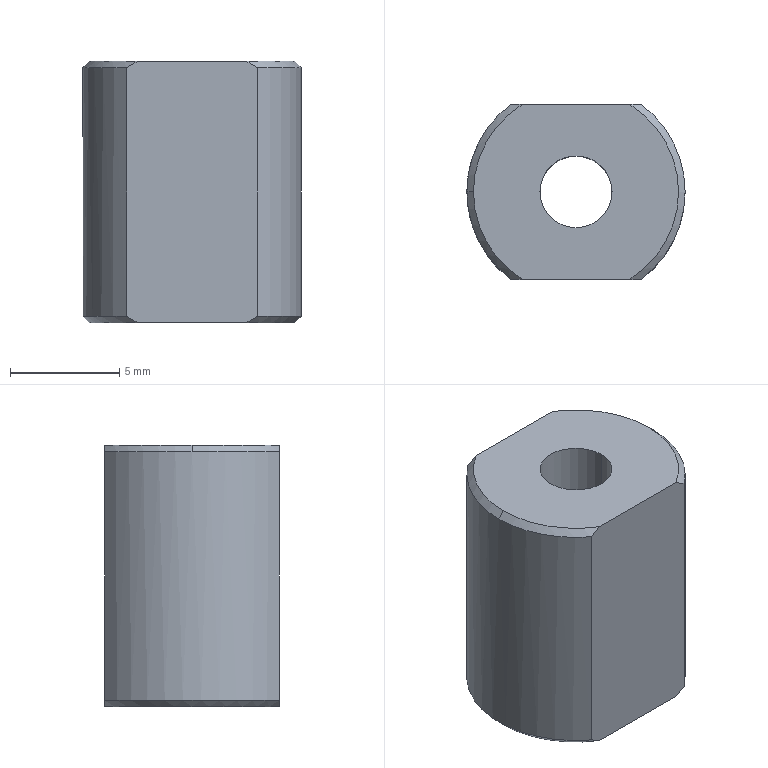Part | NX | 1 solid | 17 faces | box 10 x 8 x 12 mm | volume 738.555 mm3 | cone 8 | cylinder 5 | plane 4 | commonest cylinder face diameters 10 x3 3.3 x2
STEP:
#1=CARTESIAN_POINT('',(5.,0.,39.2));
#2=VERTEX_POINT('',#1);
#3=CARTESIAN_POINT('',(5.,0.,50.6));
#4=VERTEX_POINT('',#3);
#5=CARTESIAN_POINT('',(5.,0.,38.9));
#6=DIRECTION('',(0.,0.,1.));
#7=VECTOR('',#6,1000.);
#8=LINE('',#5,#7);
#9=EDGE_CURVE('',#2,#4,#8,.T.);
#10=ORIENTED_EDGE('',*,*,#9,.F.);
#11=CARTESIAN_POINT('',(3.,4.,39.2));
#12=VERTEX_POINT('',#11);
#13=CARTESIAN_POINT('',(0.,0.,39.2));
#14=DIRECTION('',(0.,0.,1.));
#15=DIRECTION('',(1.,0.,0.));
#16=AXIS2_PLACEMENT_3D('',#13,#14,#15);
#17=CIRCLE('',#16,5.);
#18=EDGE_CURVE('',#2,#12,#17,.T.);
#19=ORIENTED_EDGE('',*,*,#18,.T.);
#20=CARTESIAN_POINT('',(3.,4.,50.6));
#21=VERTEX_POINT('',#20);
#22=CARTESIAN_POINT('',(3.,4.,38.9));
#23=DIRECTION('',(0.,0.,1.));
#24=VECTOR('',#23,1000.);
#25=LINE('',#22,#24);
#26=EDGE_CURVE('',#12,#21,#25,.T.);
#27=ORIENTED_EDGE('',*,*,#26,.T.);
#28=CARTESIAN_POINT('',(0.,0.,50.6));
#29=DIRECTION('',(0.,0.,1.));
#30=DIRECTION('',(1.,0.,0.));
#31=AXIS2_PLACEMENT_3D('',#28,#29,#30);
#32=CIRCLE('',#31,5.);
#33=EDGE_CURVE('',#4,#21,#32,.T.);
#34=ORIENTED_EDGE('',*,*,#33,.F.);
#35=EDGE_LOOP('',(#10,#19,#27,#34));
#36=FACE_BOUND('',#35,.T.);
#37=CARTESIAN_POINT('',(0.,0.,38.9));
#38=DIRECTION('',(0.,0.,1.));
#39=DIRECTION('',(1.,0.,0.));
#40=AXIS2_PLACEMENT_3D('',#37,#38,#39);
#41=CYLINDRICAL_SURFACE('',#40,5.);
#42=ADVANCED_FACE('',(#36),#41,.T.);
#43=CARTESIAN_POINT('',(-3.,-4.,39.2));
#44=VERTEX_POINT('',#43);
#45=CARTESIAN_POINT('',(-3.,-4.,50.6));
#46=VERTEX_POINT('',#45);
#47=CARTESIAN_POINT('',(-3.,-4.,38.9));
#48=DIRECTION('',(0.,0.,1.));
#49=VECTOR('',#48,1000.);
#50=LINE('',#47,#49);
#51=EDGE_CURVE('',#44,#46,#50,.T.);
#52=ORIENTED_EDGE('',*,*,#51,.T.);
#53=CARTESIAN_POINT('',(-5.,0.,50.6));
#54=VERTEX_POINT('',#53);
#55=CARTESIAN_POINT('',(0.,0.,50.6));
#56=DIRECTION('',(0.,0.,1.));
#57=DIRECTION('',(1.,0.,0.));
#58=AXIS2_PLACEMENT_3D('',#55,#56,#57);
#59=CIRCLE('',#58,5.);
#60=EDGE_CURVE('',#54,#46,#59,.T.);
#61=ORIENTED_EDGE('',*,*,#60,.F.);
#62=CARTESIAN_POINT('',(-3.,4.,50.6));
#63=VERTEX_POINT('',#62);
#64=CARTESIAN_POINT('',(0.,0.,50.6));
#65=DIRECTION('',(0.,0.,1.));
#66=DIRECTION('',(1.,0.,0.));
#67=AXIS2_PLACEMENT_3D('',#64,#65,#66);
#68=CIRCLE('',#67,5.);
#69=EDGE_CURVE('',#63,#54,#68,.T.);
#70=ORIENTED_EDGE('',*,*,#69,.F.);
#71=CARTESIAN_POINT('',(-3.,4.,39.2));
#72=VERTEX_POINT('',#71);
#73=CARTESIAN_POINT('',(-3.,4.,38.9));
#74=DIRECTION('',(0.,0.,1.));
#75=VECTOR('',#74,1000.);
#76=LINE('',#73,#75);
#77=EDGE_CURVE('',#72,#63,#76,.T.);
#78=ORIENTED_EDGE('',*,*,#77,.F.);
#79=CARTESIAN_POINT('',(0.,0.,39.2));
#80=DIRECTION('',(0.,0.,1.));
#81=DIRECTION('',(1.,0.,0.));
#82=AXIS2_PLACEMENT_3D('',#79,#80,#81);
#83=CIRCLE('',#82,5.);
#84=EDGE_CURVE('',#72,#44,#83,.T.);
#85=ORIENTED_EDGE('',*,*,#84,.T.);
#86=EDGE_LOOP('',(#52,#61,#70,#78,#85));
#87=FACE_BOUND('',#86,.T.);
#88=CARTESIAN_POINT('',(0.,0.,38.9));
#89=DIRECTION('',(0.,0.,1.));
#90=DIRECTION('',(1.,0.,0.));
#91=AXIS2_PLACEMENT_3D('',#88,#89,#90);
#92=CYLINDRICAL_SURFACE('',#91,5.);
#93=ADVANCED_FACE('',(#87),#92,.T.);
#94=CARTESIAN_POINT('',(2.468,-4.,50.9));
#95=VERTEX_POINT('',#94);
#96=CARTESIAN_POINT('',(2.468,4.,50.9));
#97=VERTEX_POINT('',#96);
#98=CARTESIAN_POINT('',(0.,0.,50.9));
#99=DIRECTION('',(0.,0.,1.));
#100=DIRECTION('',(1.,0.,0.));
#101=AXIS2_PLACEMENT_3D('',#98,#99,#100);
#102=CIRCLE('',#101,4.7);
#103=EDGE_CURVE('',#95,#97,#102,.T.);
#104=ORIENTED_EDGE('',*,*,#103,.T.);
#105=CARTESIAN_POINT('',(-2.468,4.,50.9));
#106=VERTEX_POINT('',#105);
#107=CARTESIAN_POINT('',(-2.871,4.,50.9));
#108=DIRECTION('',(1.,0.,0.));
#109=VECTOR('',#108,1000.);
#110=LINE('',#107,#109);
#111=EDGE_CURVE('',#106,#97,#110,.T.);
#112=ORIENTED_EDGE('',*,*,#111,.F.);
#113=CARTESIAN_POINT('',(-4.7,0.,50.9));
#114=VERTEX_POINT('',#113);
#115=CARTESIAN_POINT('',(0.,0.,50.9));
#116=DIRECTION('',(0.,0.,1.));
#117=DIRECTION('',(1.,0.,0.));
#118=AXIS2_PLACEMENT_3D('',#115,#116,#117);
#119=CIRCLE('',#118,4.7);
#120=EDGE_CURVE('',#106,#114,#119,.T.);
#121=ORIENTED_EDGE('',*,*,#120,.T.);
#122=CARTESIAN_POINT('',(-2.468,-4.,50.9));
#123=VERTEX_POINT('',#122);
#124=CARTESIAN_POINT('',(0.,0.,50.9));
#125=DIRECTION('',(0.,0.,1.));
#126=DIRECTION('',(1.,0.,0.));
#127=AXIS2_PLACEMENT_3D('',#124,#125,#126);
#128=CIRCLE('',#127,4.7);
#129=EDGE_CURVE('',#114,#123,#128,.T.);
#130=ORIENTED_EDGE('',*,*,#129,.T.);
#131=CARTESIAN_POINT('',(-2.871,-4.,50.9));
#132=DIRECTION('',(-1.,0.,0.));
#133=VECTOR('',#132,1000.);
#134=LINE('',#131,#133);
#135=EDGE_CURVE('',#95,#123,#134,.T.);
#136=ORIENTED_EDGE('',*,*,#135,.F.);
#137=EDGE_LOOP('',(#104,#112,#121,#130,#136));
#138=FACE_BOUND('',#137,.T.);
#139=CARTESIAN_POINT('',(1.65,0.,50.9));
#140=VERTEX_POINT('',#139);
#141=CARTESIAN_POINT('',(-1.65,0.,50.9));
#142=VERTEX_POINT('',#141);
#143=CARTESIAN_POINT('',(0.,0.,50.9));
#144=DIRECTION('',(0.,0.,-1.));
#145=DIRECTION('',(-1.,0.,0.));
#146=AXIS2_PLACEMENT_3D('',#143,#144,#145);
#147=CIRCLE('',#146,1.65);
#148=EDGE_CURVE('',#140,#142,#147,.T.);
#149=ORIENTED_EDGE('',*,*,#148,.T.);
#150=CARTESIAN_POINT('',(0.,0.,50.9));
#151=DIRECTION('',(0.,0.,-1.));
#152=DIRECTION('',(-1.,0.,0.));
#153=AXIS2_PLACEMENT_3D('',#150,#151,#152);
#154=CIRCLE('',#153,1.65);
#155=EDGE_CURVE('',#142,#140,#154,.T.);
#156=ORIENTED_EDGE('',*,*,#155,.T.);
#157=EDGE_LOOP('',(#149,#156));
#158=FACE_BOUND('',#157,.T.);
#159=CARTESIAN_POINT('',(-2.871,0.,50.9));
#160=DIRECTION('',(0.,0.,1.));
#161=DIRECTION('',(1.,0.,0.));
#162=AXIS2_PLACEMENT_3D('',#159,#160,#161);
#163=PLANE('',#162);
#164=ADVANCED_FACE('',(#138,#158),#163,.T.);
#165=CARTESIAN_POINT('',(1.65,0.,39.284));
#166=VERTEX_POINT('',#165);
#167=CARTESIAN_POINT('',(-1.65,0.,39.284));
#168=VERTEX_POINT('',#167);
#169=CARTESIAN_POINT('',(0.,0.,39.284));
#170=DIRECTION('',(0.,0.,-1.));
#171=DIRECTION('',(-1.,0.,0.));
#172=AXIS2_PLACEMENT_3D('',#169,#170,#171);
#173=CIRCLE('',#172,1.65);
#174=EDGE_CURVE('',#166,#168,#173,.T.);
#175=ORIENTED_EDGE('',*,*,#174,.T.);
#176=CARTESIAN_POINT('',(-1.65,0.,38.9));
#177=DIRECTION('',(0.,0.,-1.));
#178=VECTOR('',#177,1000.);
#179=LINE('',#176,#178);
#180=EDGE_CURVE('',#168,#142,#179,.F.);
#181=ORIENTED_EDGE('',*,*,#180,.T.);
#182=ORIENTED_EDGE('',*,*,#148,.F.);
#183=CARTESIAN_POINT('',(1.65,0.,38.9));
#184=DIRECTION('',(0.,0.,-1.));
#185=VECTOR('',#184,1000.);
#186=LINE('',#183,#185);
#187=EDGE_CURVE('',#166,#140,#186,.F.);
#188=ORIENTED_EDGE('',*,*,#187,.F.);
#189=EDGE_LOOP('',(#175,#181,#182,#188));
#190=FACE_BOUND('',#189,.T.);
#191=CARTESIAN_POINT('',(0.,0.,38.9));
#192=DIRECTION('',(0.,0.,-1.));
#193=DIRECTION('',(-1.,0.,0.));
#194=AXIS2_PLACEMENT_3D('',#191,#192,#193);
#195=CYLINDRICAL_SURFACE('',#194,1.65);
#196=ADVANCED_FACE('',(#190),#195,.F.);
#197=ORIENTED_EDGE('',*,*,#174,.F.);
#198=CARTESIAN_POINT('',(2.315,0.,38.9));
#199=VERTEX_POINT('',#198);
#200=CARTESIAN_POINT('',(1.65,0.,39.284));
#201=DIRECTION('',(0.866,0.,-0.5));
#202=VECTOR('',#201,1000.);
#203=LINE('',#200,#202);
#204=EDGE_CURVE('',#199,#166,#203,.F.);
#205=ORIENTED_EDGE('',*,*,#204,.F.);
#206=CARTESIAN_POINT('',(-2.315,0.,38.9));
#207=VERTEX_POINT('',#206);
#208=CARTESIAN_POINT('',(0.,0.,38.9));
#209=DIRECTION('',(0.,0.,-1.));
#210=DIRECTION('',(-1.,0.,0.));
#211=AXIS2_PLACEMENT_3D('',#208,#209,#210);
#212=CIRCLE('',#211,2.315);
#213=EDGE_CURVE('',#199,#207,#212,.T.);
#214=ORIENTED_EDGE('',*,*,#213,.T.);
#215=CARTESIAN_POINT('',(-1.65,0.,39.284));
#216=DIRECTION('',(-0.866,0.,-0.5));
#217=VECTOR('',#216,1000.);
#218=LINE('',#215,#217);
#219=EDGE_CURVE('',#207,#168,#218,.F.);
#220=ORIENTED_EDGE('',*,*,#219,.T.);
#221=EDGE_LOOP('',(#197,#205,#214,#220));
#222=FACE_BOUND('',#221,.T.);
#223=CARTESIAN_POINT('',(0.,0.,39.284));
#224=DIRECTION('',(0.,0.,-1.));
#225=DIRECTION('',(-1.,0.,0.));
#226=AXIS2_PLACEMENT_3D('',#223,#224,#225);
#227=CONICAL_SURFACE('',#226,1.65,1.047);
#228=ADVANCED_FACE('',(#222),#227,.F.);
#229=ORIENTED_EDGE('',*,*,#51,.F.);
#230=CARTESIAN_POINT('',(-2.468,-4.,38.9));
#231=VERTEX_POINT('',#230);
#232=CARTESIAN_POINT('',(-3.,-4.,39.2));
#233=CARTESIAN_POINT('',(-2.956,-4.,39.174));
#234=CARTESIAN_POINT('',(-2.913,-4.,39.148));
#235=CARTESIAN_POINT('',(-2.869,-4.,39.122));
#236=CARTESIAN_POINT('',(-2.825,-4.,39.097));
#237=CARTESIAN_POINT('',(-2.781,-4.,39.071));
#238=CARTESIAN_POINT('',(-2.736,-4.,39.046));
#239=CARTESIAN_POINT('',(-2.692,-4.,39.021));
#240=CARTESIAN_POINT('',(-2.647,-4.,38.997));
#241=CARTESIAN_POINT('',(-2.603,-4.,38.972));
#242=CARTESIAN_POINT('',(-2.558,-4.,38.948));
#243=CARTESIAN_POINT('',(-2.513,-4.,38.924));
#244=CARTESIAN_POINT('',(-2.468,-4.,38.9));
#245=B_SPLINE_CURVE_WITH_KNOTS('',3,(#232,#233,#234,#235,#236,#237,#238,#239,#240,#241,#242,#243,#244),.UNSPECIFIED.,.F.,.F.,(4,3,3,3,4),(0.,0.1525,0.3051,0.458,0.611),.UNSPECIFIED.);
#246=EDGE_CURVE('',#44,#231,#245,.T.);
#247=ORIENTED_EDGE('',*,*,#246,.T.);
#248=CARTESIAN_POINT('',(2.468,-4.,38.9));
#249=VERTEX_POINT('',#248);
#250=CARTESIAN_POINT('',(-2.871,-4.,38.9));
#251=DIRECTION('',(-1.,0.,0.));
#252=VECTOR('',#251,1000.);
#253=LINE('',#250,#252);
#254=EDGE_CURVE('',#249,#231,#253,.T.);
#255=ORIENTED_EDGE('',*,*,#254,.F.);
#256=CARTESIAN_POINT('',(3.,-4.,39.2));
#257=VERTEX_POINT('',#256);
#258=CARTESIAN_POINT('',(2.468,-4.,38.9));
#259=CARTESIAN_POINT('',(2.513,-4.,38.924));
#260=CARTESIAN_POINT('',(2.558,-4.,38.948));
#261=CARTESIAN_POINT('',(2.602,-4.,38.972));
#262=CARTESIAN_POINT('',(2.647,-4.,38.996));
#263=CARTESIAN_POINT('',(2.692,-4.,39.021));
#264=CARTESIAN_POINT('',(2.736,-4.,39.046));
#265=CARTESIAN_POINT('',(2.78,-4.,39.071));
#266=CARTESIAN_POINT('',(2.824,-4.,39.097));
#267=CARTESIAN_POINT('',(2.868,-4.,39.122));
#268=CARTESIAN_POINT('',(2.912,-4.,39.148));
#269=CARTESIAN_POINT('',(2.956,-4.,39.174));
#270=CARTESIAN_POINT('',(3.,-4.,39.2));
#271=B_SPLINE_CURVE_WITH_KNOTS('',3,(#258,#259,#260,#261,#262,#263,#264,#265,#266,#267,#268,#269,#270),.UNSPECIFIED.,.F.,.F.,(4,3,3,3,4),(0.,0.1527,0.3054,0.4582,0.611),.UNSPECIFIED.);
#272=EDGE_CURVE('',#249,#257,#271,.T.);
#273=ORIENTED_EDGE('',*,*,#272,.T.);
#274=CARTESIAN_POINT('',(3.,-4.,50.6));
#275=VERTEX_POINT('',#274);
#276=CARTESIAN_POINT('',(3.,-4.,38.9));
#277=DIRECTION('',(0.,0.,1.));
#278=VECTOR('',#277,1000.);
#279=LINE('',#276,#278);
#280=EDGE_CURVE('',#257,#275,#279,.T.);
#281=ORIENTED_EDGE('',*,*,#280,.T.);
#282=CARTESIAN_POINT('',(3.,-4.,50.6));
#283=CARTESIAN_POINT('',(2.956,-4.,50.626));
#284=CARTESIAN_POINT('',(2.912,-4.,50.652));
#285=CARTESIAN_POINT('',(2.868,-4.,50.678));
#286=CARTESIAN_POINT('',(2.824,-4.,50.703));
#287=CARTESIAN_POINT('',(2.78,-4.,50.729));
#288=CARTESIAN_POINT('',(2.736,-4.,50.754));
#289=CARTESIAN_POINT('',(2.692,-4.,50.779));
#290=CARTESIAN_POINT('',(2.647,-4.,50.804));
#291=CARTESIAN_POINT('',(2.602,-4.,50.828));
#292=CARTESIAN_POINT('',(2.558,-4.,50.852));
#293=CARTESIAN_POINT('',(2.513,-4.,50.876));
#294=CARTESIAN_POINT('',(2.468,-4.,50.9));
#295=B_SPLINE_CURVE_WITH_KNOTS('',3,(#282,#283,#284,#285,#286,#287,#288,#289,#290,#291,#292,#293,#294),.UNSPECIFIED.,.F.,.F.,(4,3,3,3,4),(0.,0.1528,0.3056,0.4583,0.611),.UNSPECIFIED.);
#296=EDGE_CURVE('',#275,#95,#295,.T.);
#297=ORIENTED_EDGE('',*,*,#296,.T.);
#298=ORIENTED_EDGE('',*,*,#135,.T.);
#299=CARTESIAN_POINT('',(-2.468,-4.,50.9));
#300=CARTESIAN_POINT('',(-2.513,-4.,50.876));
#301=CARTESIAN_POINT('',(-2.558,-4.,50.852));
#302=CARTESIAN_POINT('',(-2.603,-4.,50.828));
#303=CARTESIAN_POINT('',(-2.647,-4.,50.803));
#304=CARTESIAN_POINT('',(-2.692,-4.,50.779));
#305=CARTESIAN_POINT('',(-2.736,-4.,50.754));
#306=CARTESIAN_POINT('',(-2.781,-4.,50.729));
#307=CARTESIAN_POINT('',(-2.825,-4.,50.703));
#308=CARTESIAN_POINT('',(-2.869,-4.,50.678));
#309=CARTESIAN_POINT('',(-2.913,-4.,50.652));
#310=CARTESIAN_POINT('',(-2.956,-4.,50.626));
#311=CARTESIAN_POINT('',(-3.,-4.,50.6));
#312=B_SPLINE_CURVE_WITH_KNOTS('',3,(#299,#300,#301,#302,#303,#304,#305,#306,#307,#308,#309,#310,#311),.UNSPECIFIED.,.F.,.F.,(4,3,3,3,4),(0.,0.153,0.3057,0.4584,0.611),.UNSPECIFIED.);
#313=EDGE_CURVE('',#123,#46,#312,.T.);
#314=ORIENTED_EDGE('',*,*,#313,.T.);
#315=EDGE_LOOP('',(#229,#247,#255,#273,#281,#297,#298,#314));
#316=FACE_BOUND('',#315,.T.);
#317=CARTESIAN_POINT('',(7.4,-4.,52.1));
#318=DIRECTION('',(0.,1.,0.));
#319=DIRECTION('',(1.,0.,0.));
#320=AXIS2_PLACEMENT_3D('',#317,#318,#319);
#321=PLANE('',#320);
#322=ADVANCED_FACE('',(#316),#321,.F.);
#323=ORIENTED_EDGE('',*,*,#26,.F.);
#324=CARTESIAN_POINT('',(2.468,4.,38.9));
#325=VERTEX_POINT('',#324);
#326=CARTESIAN_POINT('',(3.,4.,39.2));
#327=CARTESIAN_POINT('',(2.956,4.,39.174));
#328=CARTESIAN_POINT('',(2.913,4.,39.148));
#329=CARTESIAN_POINT('',(2.869,4.,39.122));
#330=CARTESIAN_POINT('',(2.825,4.,39.097));
#331=CARTESIAN_POINT('',(2.781,4.,39.071));
#332=CARTESIAN_POINT('',(2.736,4.,39.046));
#333=CARTESIAN_POINT('',(2.692,4.,39.021));
#334=CARTESIAN_POINT('',(2.647,4.,38.997));
#335=CARTESIAN_POINT('',(2.603,4.,38.972));
#336=CARTESIAN_POINT('',(2.558,4.,38.948));
#337=CARTESIAN_POINT('',(2.513,4.,38.924));
#338=CARTESIAN_POINT('',(2.468,4.,38.9));
#339=B_SPLINE_CURVE_WITH_KNOTS('',3,(#326,#327,#328,#329,#330,#331,#332,#333,#334,#335,#336,#337,#338),.UNSPECIFIED.,.F.,.F.,(4,3,3,3,4),(0.,0.1525,0.3051,0.458,0.611),.UNSPECIFIED.);
#340=EDGE_CURVE('',#12,#325,#339,.T.);
#341=ORIENTED_EDGE('',*,*,#340,.T.);
#342=CARTESIAN_POINT('',(-2.468,4.,38.9));
#343=VERTEX_POINT('',#342);
#344=CARTESIAN_POINT('',(-2.871,4.,38.9));
#345=DIRECTION('',(1.,0.,0.));
#346=VECTOR('',#345,1000.);
#347=LINE('',#344,#346);
#348=EDGE_CURVE('',#343,#325,#347,.T.);
#349=ORIENTED_EDGE('',*,*,#348,.F.);
#350=CARTESIAN_POINT('',(-2.468,4.,38.9));
#351=CARTESIAN_POINT('',(-2.513,4.,38.924));
#352=CARTESIAN_POINT('',(-2.558,4.,38.948));
#353=CARTESIAN_POINT('',(-2.602,4.,38.972));
#354=CARTESIAN_POINT('',(-2.647,4.,38.996));
#355=CARTESIAN_POINT('',(-2.692,4.,39.021));
#356=CARTESIAN_POINT('',(-2.736,4.,39.046));
#357=CARTESIAN_POINT('',(-2.78,4.,39.071));
#358=CARTESIAN_POINT('',(-2.824,4.,39.097));
#359=CARTESIAN_POINT('',(-2.868,4.,39.122));
#360=CARTESIAN_POINT('',(-2.912,4.,39.148));
#361=CARTESIAN_POINT('',(-2.956,4.,39.174));
#362=CARTESIAN_POINT('',(-3.,4.,39.2));
#363=B_SPLINE_CURVE_WITH_KNOTS('',3,(#350,#351,#352,#353,#354,#355,#356,#357,#358,#359,#360,#361,#362),.UNSPECIFIED.,.F.,.F.,(4,3,3,3,4),(0.,0.1527,0.3054,0.4582,0.611),.UNSPECIFIED.);
#364=EDGE_CURVE('',#343,#72,#363,.T.);
#365=ORIENTED_EDGE('',*,*,#364,.T.);
#366=ORIENTED_EDGE('',*,*,#77,.T.);
#367=CARTESIAN_POINT('',(-3.,4.,50.6));
#368=CARTESIAN_POINT('',(-2.956,4.,50.626));
#369=CARTESIAN_POINT('',(-2.912,4.,50.652));
#370=CARTESIAN_POINT('',(-2.868,4.,50.678));
#371=CARTESIAN_POINT('',(-2.824,4.,50.703));
#372=CARTESIAN_POINT('',(-2.78,4.,50.729));
#373=CARTESIAN_POINT('',(-2.736,4.,50.754));
#374=CARTESIAN_POINT('',(-2.692,4.,50.779));
#375=CARTESIAN_POINT('',(-2.647,4.,50.804));
#376=CARTESIAN_POINT('',(-2.602,4.,50.828));
#377=CARTESIAN_POINT('',(-2.558,4.,50.852));
#378=CARTESIAN_POINT('',(-2.513,4.,50.876));
#379=CARTESIAN_POINT('',(-2.468,4.,50.9));
#380=B_SPLINE_CURVE_WITH_KNOTS('',3,(#367,#368,#369,#370,#371,#372,#373,#374,#375,#376,#377,#378,#379),.UNSPECIFIED.,.F.,.F.,(4,3,3,3,4),(0.,0.1528,0.3056,0.4583,0.611),.UNSPECIFIED.);
#381=EDGE_CURVE('',#63,#106,#380,.T.);
#382=ORIENTED_EDGE('',*,*,#381,.T.);
#383=ORIENTED_EDGE('',*,*,#111,.T.);
#384=CARTESIAN_POINT('',(2.468,4.,50.9));
#385=CARTESIAN_POINT('',(2.513,4.,50.876));
#386=CARTESIAN_POINT('',(2.558,4.,50.852));
#387=CARTESIAN_POINT('',(2.603,4.,50.828));
#388=CARTESIAN_POINT('',(2.647,4.,50.803));
#389=CARTESIAN_POINT('',(2.692,4.,50.779));
#390=CARTESIAN_POINT('',(2.736,4.,50.754));
#391=CARTESIAN_POINT('',(2.781,4.,50.729));
#392=CARTESIAN_POINT('',(2.825,4.,50.703));
#393=CARTESIAN_POINT('',(2.869,4.,50.678));
#394=CARTESIAN_POINT('',(2.913,4.,50.652));
#395=CARTESIAN_POINT('',(2.956,4.,50.626));
#396=CARTESIAN_POINT('',(3.,4.,50.6));
#397=B_SPLINE_CURVE_WITH_KNOTS('',3,(#384,#385,#386,#387,#388,#389,#390,#391,#392,#393,#394,#395,#396),.UNSPECIFIED.,.F.,.F.,(4,3,3,3,4),(0.,0.153,0.3058,0.4584,0.611),.UNSPECIFIED.);
#398=EDGE_CURVE('',#97,#21,#397,.T.);
#399=ORIENTED_EDGE('',*,*,#398,.T.);
#400=EDGE_LOOP('',(#323,#341,#349,#365,#366,#382,#383,#399));
#401=FACE_BOUND('',#400,.T.);
#402=CARTESIAN_POINT('',(-5.9,4.,52.1));
#403=DIRECTION('',(0.,-1.,0.));
#404=DIRECTION('',(0.,0.,-1.));
#405=AXIS2_PLACEMENT_3D('',#402,#403,#404);
#406=PLANE('',#405);
#407=ADVANCED_FACE('',(#401),#406,.F.);
#408=CARTESIAN_POINT('',(-4.7,0.,50.9));
#409=DIRECTION('',(-0.7071,0.,-0.7071));
#410=VECTOR('',#409,1000.);
#411=LINE('',#408,#410);
#412=EDGE_CURVE('',#114,#54,#411,.T.);
#413=ORIENTED_EDGE('',*,*,#412,.F.);
#414=ORIENTED_EDGE('',*,*,#120,.F.);
#415=ORIENTED_EDGE('',*,*,#381,.F.);
#416=ORIENTED_EDGE('',*,*,#69,.T.);
#417=EDGE_LOOP('',(#413,#414,#415,#416));
#418=FACE_BOUND('',#417,.T.);
#419=CARTESIAN_POINT('',(0.,0.,50.9));
#420=DIRECTION('',(0.,0.,-1.));
#421=DIRECTION('',(-1.,0.,0.));
#422=AXIS2_PLACEMENT_3D('',#419,#420,#421);
#423=CONICAL_SURFACE('',#422,4.7,0.7854);
#424=ADVANCED_FACE('',(#418),#423,.T.);
#425=ORIENTED_EDGE('',*,*,#103,.F.);
#426=ORIENTED_EDGE('',*,*,#296,.F.);
#427=CARTESIAN_POINT('',(0.,0.,50.6));
#428=DIRECTION('',(0.,0.,1.));
#429=DIRECTION('',(1.,0.,0.));
#430=AXIS2_PLACEMENT_3D('',#427,#428,#429);
#431=CIRCLE('',#430,5.);
#432=EDGE_CURVE('',#275,#4,#431,.T.);
#433=ORIENTED_EDGE('',*,*,#432,.T.);
#434=ORIENTED_EDGE('',*,*,#33,.T.);
#435=ORIENTED_EDGE('',*,*,#398,.F.);
#436=EDGE_LOOP('',(#425,#426,#433,#434,#435));
#437=FACE_BOUND('',#436,.T.);
#438=CARTESIAN_POINT('',(0.,0.,50.9));
#439=DIRECTION('',(0.,0.,-1.));
#440=DIRECTION('',(-1.,0.,0.));
#441=AXIS2_PLACEMENT_3D('',#438,#439,#440);
#442=CONICAL_SURFACE('',#441,4.7,0.7854);
#443=ADVANCED_FACE('',(#437),#442,.T.);
#444=ORIENTED_EDGE('',*,*,#180,.F.);
#445=CARTESIAN_POINT('',(0.,0.,39.284));
#446=DIRECTION('',(0.,0.,-1.));
#447=DIRECTION('',(-1.,0.,0.));
#448=AXIS2_PLACEMENT_3D('',#445,#446,#447);
#449=CIRCLE('',#448,1.65);
#450=EDGE_CURVE('',#168,#166,#449,.T.);
#451=ORIENTED_EDGE('',*,*,#450,.T.);
#452=ORIENTED_EDGE('',*,*,#187,.T.);
#453=ORIENTED_EDGE('',*,*,#155,.F.);
#454=EDGE_LOOP('',(#444,#451,#452,#453));
#455=FACE_BOUND('',#454,.T.);
#456=CARTESIAN_POINT('',(0.,0.,38.9));
#457=DIRECTION('',(0.,0.,-1.));
#458=DIRECTION('',(-1.,0.,0.));
#459=AXIS2_PLACEMENT_3D('',#456,#457,#458);
#460=CYLINDRICAL_SURFACE('',#459,1.65);
#461=ADVANCED_FACE('',(#455),#460,.F.);
#462=ORIENTED_EDGE('',*,*,#219,.F.);
#463=CARTESIAN_POINT('',(0.,0.,38.9));
#464=DIRECTION('',(0.,0.,-1.));
#465=DIRECTION('',(-1.,0.,0.));
#466=AXIS2_PLACEMENT_3D('',#463,#464,#465);
#467=CIRCLE('',#466,2.315);
#468=EDGE_CURVE('',#207,#199,#467,.T.);
#469=ORIENTED_EDGE('',*,*,#468,.T.);
#470=ORIENTED_EDGE('',*,*,#204,.T.);
#471=ORIENTED_EDGE('',*,*,#450,.F.);
#472=EDGE_LOOP('',(#462,#469,#470,#471));
#473=FACE_BOUND('',#472,.T.);
#474=CARTESIAN_POINT('',(0.,0.,39.284));
#475=DIRECTION('',(0.,0.,-1.));
#476=DIRECTION('',(-1.,0.,0.));
#477=AXIS2_PLACEMENT_3D('',#474,#475,#476);
#478=CONICAL_SURFACE('',#477,1.65,1.047);
#479=ADVANCED_FACE('',(#473),#478,.F.);
#480=CARTESIAN_POINT('',(0.,0.,38.9));
#481=DIRECTION('',(0.,0.,1.));
#482=DIRECTION('',(1.,0.,0.));
#483=AXIS2_PLACEMENT_3D('',#480,#481,#482);
#484=CIRCLE('',#483,4.7);
#485=EDGE_CURVE('',#343,#231,#484,.T.);
#486=ORIENTED_EDGE('',*,*,#485,.F.);
#487=ORIENTED_EDGE('',*,*,#348,.T.);
#488=CARTESIAN_POINT('',(4.7,0.,38.9));
#489=VERTEX_POINT('',#488);
#490=CARTESIAN_POINT('',(0.,0.,38.9));
#491=DIRECTION('',(0.,0.,1.));
#492=DIRECTION('',(1.,0.,0.));
#493=AXIS2_PLACEMENT_3D('',#490,#491,#492);
#494=CIRCLE('',#493,4.7);
#495=EDGE_CURVE('',#489,#325,#494,.T.);
#496=ORIENTED_EDGE('',*,*,#495,.F.);
#497=CARTESIAN_POINT('',(0.,0.,38.9));
#498=DIRECTION('',(0.,0.,1.));
#499=DIRECTION('',(1.,0.,0.));
#500=AXIS2_PLACEMENT_3D('',#497,#498,#499);
#501=CIRCLE('',#500,4.7);
#502=EDGE_CURVE('',#249,#489,#501,.T.);
#503=ORIENTED_EDGE('',*,*,#502,.F.);
#504=ORIENTED_EDGE('',*,*,#254,.T.);
#505=EDGE_LOOP('',(#486,#487,#496,#503,#504));
#506=FACE_BOUND('',#505,.T.);
#507=ORIENTED_EDGE('',*,*,#213,.F.);
#508=ORIENTED_EDGE('',*,*,#468,.F.);
#509=EDGE_LOOP('',(#507,#508));
#510=FACE_BOUND('',#509,.T.);
#511=CARTESIAN_POINT('',(-2.871,0.,38.9));
#512=DIRECTION('',(0.,0.,1.));
#513=DIRECTION('',(1.,0.,0.));
#514=AXIS2_PLACEMENT_3D('',#511,#512,#513);
#515=PLANE('',#514);
#516=ADVANCED_FACE('',(#506,#510),#515,.F.);
#517=CARTESIAN_POINT('',(4.7,0.,38.9));
#518=DIRECTION('',(0.7071,0.,0.7071));
#519=VECTOR('',#518,1000.);
#520=LINE('',#517,#519);
#521=EDGE_CURVE('',#489,#2,#520,.T.);
#522=ORIENTED_EDGE('',*,*,#521,.F.);
#523=ORIENTED_EDGE('',*,*,#495,.T.);
#524=ORIENTED_EDGE('',*,*,#340,.F.);
#525=ORIENTED_EDGE('',*,*,#18,.F.);
#526=EDGE_LOOP('',(#522,#523,#524,#525));
#527=FACE_BOUND('',#526,.T.);
#528=CARTESIAN_POINT('',(0.,0.,38.9));
#529=DIRECTION('',(0.,0.,1.));
#530=DIRECTION('',(1.,0.,0.));
#531=AXIS2_PLACEMENT_3D('',#528,#529,#530);
#532=CONICAL_SURFACE('',#531,4.7,0.7854);
#533=ADVANCED_FACE('',(#527),#532,.T.);
#534=ORIENTED_EDGE('',*,*,#485,.T.);
#535=ORIENTED_EDGE('',*,*,#246,.F.);
#536=ORIENTED_EDGE('',*,*,#84,.F.);
#537=ORIENTED_EDGE('',*,*,#364,.F.);
#538=EDGE_LOOP('',(#534,#535,#536,#537));
#539=FACE_BOUND('',#538,.T.);
#540=CARTESIAN_POINT('',(0.,0.,38.9));
#541=DIRECTION('',(0.,0.,1.));
#542=DIRECTION('',(1.,0.,0.));
#543=AXIS2_PLACEMENT_3D('',#540,#541,#542);
#544=CONICAL_SURFACE('',#543,4.7,0.7854);
#545=ADVANCED_FACE('',(#539),#544,.T.);
#546=ORIENTED_EDGE('',*,*,#502,.T.);
#547=ORIENTED_EDGE('',*,*,#521,.T.);
#548=CARTESIAN_POINT('',(0.,0.,39.2));
#549=DIRECTION('',(0.,0.,1.));
#550=DIRECTION('',(1.,0.,0.));
#551=AXIS2_PLACEMENT_3D('',#548,#549,#550);
#552=CIRCLE('',#551,5.);
#553=EDGE_CURVE('',#257,#2,#552,.T.);
#554=ORIENTED_EDGE('',*,*,#553,.F.);
#555=ORIENTED_EDGE('',*,*,#272,.F.);
#556=EDGE_LOOP('',(#546,#547,#554,#555));
#557=FACE_BOUND('',#556,.T.);
#558=CARTESIAN_POINT('',(0.,0.,38.9));
#559=DIRECTION('',(0.,0.,1.));
#560=DIRECTION('',(1.,0.,0.));
#561=AXIS2_PLACEMENT_3D('',#558,#559,#560);
#562=CONICAL_SURFACE('',#561,4.7,0.7854);
#563=ADVANCED_FACE('',(#557),#562,.T.);
#564=ORIENTED_EDGE('',*,*,#129,.F.);
#565=ORIENTED_EDGE('',*,*,#412,.T.);
#566=ORIENTED_EDGE('',*,*,#60,.T.);
#567=ORIENTED_EDGE('',*,*,#313,.F.);
#568=EDGE_LOOP('',(#564,#565,#566,#567));
#569=FACE_BOUND('',#568,.T.);
#570=CARTESIAN_POINT('',(0.,0.,50.9));
#571=DIRECTION('',(0.,0.,-1.));
#572=DIRECTION('',(-1.,0.,0.));
#573=AXIS2_PLACEMENT_3D('',#570,#571,#572);
#574=CONICAL_SURFACE('',#573,4.7,0.7854);
#575=ADVANCED_FACE('',(#569),#574,.T.);
#576=ORIENTED_EDGE('',*,*,#553,.T.);
#577=ORIENTED_EDGE('',*,*,#9,.T.);
#578=ORIENTED_EDGE('',*,*,#432,.F.);
#579=ORIENTED_EDGE('',*,*,#280,.F.);
#580=EDGE_LOOP('',(#576,#577,#578,#579));
#581=FACE_BOUND('',#580,.T.);
#582=CARTESIAN_POINT('',(0.,0.,38.9));
#583=DIRECTION('',(0.,0.,1.));
#584=DIRECTION('',(1.,0.,0.));
#585=AXIS2_PLACEMENT_3D('',#582,#583,#584);
#586=CYLINDRICAL_SURFACE('',#585,5.);
#587=ADVANCED_FACE('',(#581),#586,.T.);
#588=CLOSED_SHELL('',(#42,#93,#164,#196,#228,#322,#407,#424,#443,#461,#479,#516,#533,#545,#563,#575,#587));
#589=MANIFOLD_SOLID_BREP('',#588);
#590=(LENGTH_UNIT()NAMED_UNIT(*)SI_UNIT(.MILLI.,.METRE.));
#591=UNCERTAINTY_MEASURE_WITH_UNIT(LENGTH_MEASURE(0.00001),#590,'','');
#592=(NAMED_UNIT(*)PLANE_ANGLE_UNIT()SI_UNIT($,.RADIAN.));
#593=(NAMED_UNIT(*)SI_UNIT($,.STERADIAN.)SOLID_ANGLE_UNIT());
#594=(GEOMETRIC_REPRESENTATION_CONTEXT(3)GLOBAL_UNCERTAINTY_ASSIGNED_CONTEXT((#591))GLOBAL_UNIT_ASSIGNED_CONTEXT((#590,#592,#593))REPRESENTATION_CONTEXT('',''));
#595=ADVANCED_BREP_SHAPE_REPRESENTATION('',(#589),#594);